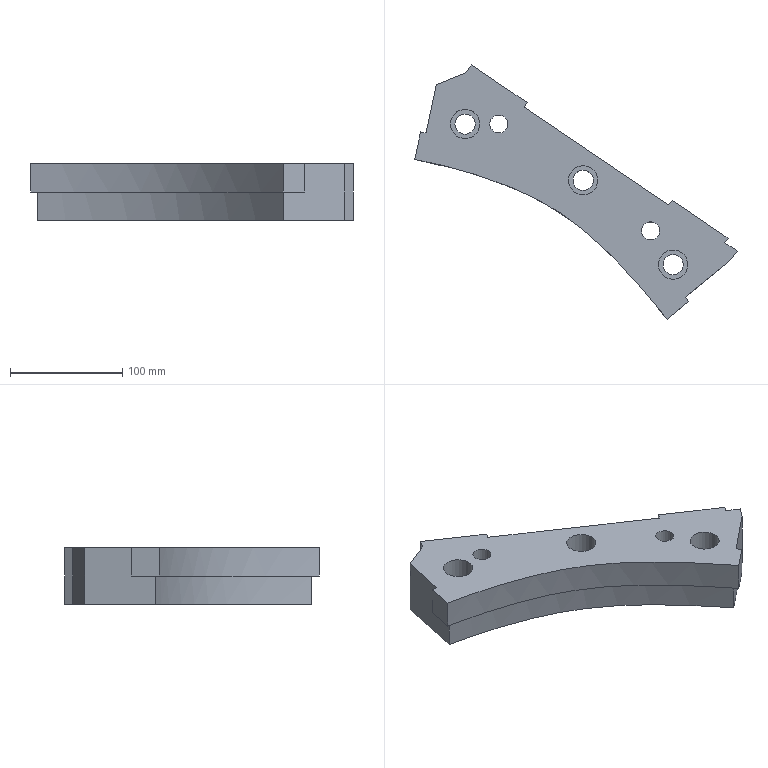Part | NX | features solid 2 | 1 solid | 32 faces | box 286.702 x 226.033 x 50 mm | volume 928298 mm3 | plane 20 | cylinder 8 | spline 4 | commonest cylinder face diameters 18 x3 26 x3 16 x2
STEP:
#1=CARTESIAN_POINT('',(-270.346,-232.178,0.));
#2=VERTEX_POINT('',#1);
#3=CARTESIAN_POINT('',(-275.25,-231.199,0.));
#4=VERTEX_POINT('',#3);
#5=CARTESIAN_POINT('',(-270.346,-232.178,0.));
#6=CARTESIAN_POINT('',(-271.979,-231.846,0.));
#7=CARTESIAN_POINT('',(-273.614,-231.52,0.));
#8=CARTESIAN_POINT('',(-275.25,-231.199,0.));
#9=B_SPLINE_CURVE_WITH_KNOTS('',3,(#5,#6,#7,#8),.UNSPECIFIED.,.F.,.F.,(4,4),(1.379,1.384),.UNSPECIFIED.);
#10=EDGE_CURVE('',#2,#4,#9,.T.);
#11=ORIENTED_EDGE('',*,*,#10,.F.);
#12=CARTESIAN_POINT('',(-270.346,-232.178,-25.));
#13=VERTEX_POINT('',#12);
#14=CARTESIAN_POINT('',(-270.346,-232.178,-25.));
#15=DIRECTION('',(0.,0.,-1.));
#16=VECTOR('',#15,1000.);
#17=LINE('',#14,#16);
#18=EDGE_CURVE('',#13,#2,#17,.F.);
#19=ORIENTED_EDGE('',*,*,#18,.F.);
#20=CARTESIAN_POINT('',(-275.25,-231.199,-25.));
#21=VERTEX_POINT('',#20);
#22=CARTESIAN_POINT('',(-270.346,-232.178,-25.));
#23=CARTESIAN_POINT('',(-271.981,-231.845,-25.));
#24=CARTESIAN_POINT('',(-273.615,-231.519,-25.));
#25=CARTESIAN_POINT('',(-275.25,-231.199,-25.));
#26=B_SPLINE_CURVE_WITH_KNOTS('',3,(#22,#23,#24,#25),.UNSPECIFIED.,.F.,.F.,(4,4),(0.9809,0.9985),.UNSPECIFIED.);
#27=EDGE_CURVE('',#13,#21,#26,.T.);
#28=ORIENTED_EDGE('',*,*,#27,.T.);
#29=CARTESIAN_POINT('',(-275.25,-231.199,-12.5));
#30=DIRECTION('',(0.,0.,-1.));
#31=VECTOR('',#30,1000.);
#32=LINE('',#29,#31);
#33=EDGE_CURVE('',#4,#21,#32,.T.);
#34=ORIENTED_EDGE('',*,*,#33,.F.);
#35=EDGE_LOOP('',(#11,#19,#28,#34));
#36=FACE_BOUND('',#35,.T.);
#37=CARTESIAN_POINT('',(-270.346,-232.178,0.));
#38=CARTESIAN_POINT('',(-270.346,-232.178,-25.));
#39=CARTESIAN_POINT('',(-271.981,-231.845,0.));
#40=CARTESIAN_POINT('',(-271.981,-231.845,-25.));
#41=CARTESIAN_POINT('',(-273.615,-231.519,0.));
#42=CARTESIAN_POINT('',(-273.615,-231.519,-25.));
#43=CARTESIAN_POINT('',(-275.25,-231.199,0.));
#44=CARTESIAN_POINT('',(-275.25,-231.199,-25.));
#45=B_SPLINE_SURFACE_WITH_KNOTS('',3,1,((#37,#38),(#39,#40),(#41,#42),(#43,#44)),.SURF_OF_LINEAR_EXTRUSION.,.F.,.F.,.F.,(4,4),(2,2),(0.9809,0.9985),(0.,1.),.PIECEWISE_BEZIER_KNOTS.);
#46=ADVANCED_FACE('',(#36),#45,.F.);
#47=CARTESIAN_POINT('',(-261.224,-189.264,-50.));
#48=VERTEX_POINT('',#47);
#49=CARTESIAN_POINT('',(-235.001,-178.669,-50.));
#50=VERTEX_POINT('',#49);
#51=CARTESIAN_POINT('',(-258.097,-188.001,-50.));
#52=DIRECTION('',(-0.9272,-0.3746,0.));
#53=VECTOR('',#52,1000.);
#54=LINE('',#51,#53);
#55=EDGE_CURVE('',#48,#50,#54,.F.);
#56=ORIENTED_EDGE('',*,*,#55,.T.);
#57=CARTESIAN_POINT('',(-230.246,-171.62,-50.));
#58=VERTEX_POINT('',#57);
#59=CARTESIAN_POINT('',(-224.654,-163.329,-50.));
#60=DIRECTION('',(0.5592,0.829,0.));
#61=VECTOR('',#60,1000.);
#62=LINE('',#59,#61);
#63=EDGE_CURVE('',#50,#58,#62,.T.);
#64=ORIENTED_EDGE('',*,*,#63,.T.);
#65=CARTESIAN_POINT('',(-180.503,-205.171,-50.));
#66=VERTEX_POINT('',#65);
#67=CARTESIAN_POINT('',(-72.1,-278.29,-50.));
#68=DIRECTION('',(0.829,-0.5592,0.));
#69=VECTOR('',#68,1000.);
#70=LINE('',#67,#69);
#71=EDGE_CURVE('',#58,#66,#70,.T.);
#72=ORIENTED_EDGE('',*,*,#71,.T.);
#73=CARTESIAN_POINT('',(-183.299,-209.317,-50.));
#74=VERTEX_POINT('',#73);
#75=CARTESIAN_POINT('',(-174.911,-196.881,-50.));
#76=DIRECTION('',(0.5592,0.829,0.));
#77=VECTOR('',#76,1000.);
#78=LINE('',#75,#77);
#79=EDGE_CURVE('',#74,#66,#78,.T.);
#80=ORIENTED_EDGE('',*,*,#79,.F.);
#81=CARTESIAN_POINT('',(-54.469,-296.214,-50.));
#82=VERTEX_POINT('',#81);
#83=CARTESIAN_POINT('',(-74.896,-282.435,-50.));
#84=DIRECTION('',(0.829,-0.5592,0.));
#85=VECTOR('',#84,1000.);
#86=LINE('',#83,#85);
#87=EDGE_CURVE('',#74,#82,#86,.T.);
#88=ORIENTED_EDGE('',*,*,#87,.T.);
#89=CARTESIAN_POINT('',(-51.673,-292.069,-50.));
#90=VERTEX_POINT('',#89);
#91=CARTESIAN_POINT('',(-46.081,-283.778,-50.));
#92=DIRECTION('',(0.5592,0.829,0.));
#93=VECTOR('',#92,1000.);
#94=LINE('',#91,#93);
#95=EDGE_CURVE('',#82,#90,#94,.T.);
#96=ORIENTED_EDGE('',*,*,#95,.T.);
#97=CARTESIAN_POINT('',(-1.931,-325.62,-50.));
#98=VERTEX_POINT('',#97);
#99=CARTESIAN_POINT('',(-72.1,-278.29,-50.));
#100=DIRECTION('',(0.829,-0.5592,0.));
#101=VECTOR('',#100,1000.);
#102=LINE('',#99,#101);
#103=EDGE_CURVE('',#90,#98,#102,.T.);
#104=ORIENTED_EDGE('',*,*,#103,.T.);
#105=CARTESIAN_POINT('',(-4.727,-329.765,-50.));
#106=VERTEX_POINT('',#105);
#107=CARTESIAN_POINT('',(3.661,-317.33,-50.));
#108=DIRECTION('',(0.5592,0.829,0.));
#109=VECTOR('',#108,1000.);
#110=LINE('',#107,#109);
#111=EDGE_CURVE('',#106,#98,#110,.T.);
#112=ORIENTED_EDGE('',*,*,#111,.F.);
#113=CARTESIAN_POINT('',(6.254,-337.172,-50.));
#114=VERTEX_POINT('',#113);
#115=CARTESIAN_POINT('',(-74.896,-282.435,-50.));
#116=DIRECTION('',(0.829,-0.5592,0.));
#117=VECTOR('',#116,1000.);
#118=LINE('',#115,#117);
#119=EDGE_CURVE('',#106,#114,#118,.T.);
#120=ORIENTED_EDGE('',*,*,#119,.T.);
#121=CARTESIAN_POINT('',(-1.187,-346.696,-50.));
#122=VERTEX_POINT('',#121);
#123=CARTESIAN_POINT('',(-528.329,-1021.407,-50.));
#124=DIRECTION('',(0.6157,0.788,0.));
#125=VECTOR('',#124,1000.);
#126=LINE('',#123,#125);
#127=EDGE_CURVE('',#122,#114,#126,.T.);
#128=ORIENTED_EDGE('',*,*,#127,.F.);
#129=CARTESIAN_POINT('',(-55.411,-390.605,-50.));
#130=VERTEX_POINT('',#129);
#131=CARTESIAN_POINT('',(-656.08,-877.018,-50.));
#132=DIRECTION('',(0.7771,0.6293,0.));
#133=VECTOR('',#132,1000.);
#134=LINE('',#131,#133);
#135=EDGE_CURVE('',#130,#122,#134,.T.);
#136=ORIENTED_EDGE('',*,*,#135,.F.);
#137=CARTESIAN_POINT('',(-274.504,-251.742,-50.));
#138=VERTEX_POINT('',#137);
#139=CARTESIAN_POINT('',(-55.411,-390.605,-50.));
#140=CARTESIAN_POINT('',(-57.422,-388.104,-50.));
#141=CARTESIAN_POINT('',(-61.329,-383.276,-50.));
#142=CARTESIAN_POINT('',(-65.923,-377.683,-50.));
#143=CARTESIAN_POINT('',(-69.426,-373.471,-50.));
#144=CARTESIAN_POINT('',(-71.964,-370.447,-50.));
#145=CARTESIAN_POINT('',(-74.015,-368.028,-50.));
#146=CARTESIAN_POINT('',(-75.397,-366.41,-50.));
#147=CARTESIAN_POINT('',(-76.201,-365.474,-50.));
#148=CARTESIAN_POINT('',(-76.728,-364.861,-50.));
#149=CARTESIAN_POINT('',(-77.518,-363.946,-50.));
#150=CARTESIAN_POINT('',(-78.477,-362.839,-50.));
#151=CARTESIAN_POINT('',(-80.191,-360.871,-50.));
#152=CARTESIAN_POINT('',(-82.598,-358.137,-50.));
#153=CARTESIAN_POINT('',(-85.465,-354.929,-50.));
#154=CARTESIAN_POINT('',(-89.243,-350.768,-50.));
#155=CARTESIAN_POINT('',(-92.968,-346.763,-50.));
#156=CARTESIAN_POINT('',(-96.153,-343.427,-50.));
#157=CARTESIAN_POINT('',(-97.989,-341.53,-50.));
#158=CARTESIAN_POINT('',(-99.27,-340.218,-50.));
#159=CARTESIAN_POINT('',(-100.882,-338.583,-50.));
#160=CARTESIAN_POINT('',(-102.912,-336.548,-50.));
#161=CARTESIAN_POINT('',(-106.509,-332.999,-50.));
#162=CARTESIAN_POINT('',(-111.59,-328.156,-50.));
#163=CARTESIAN_POINT('',(-116.654,-323.554,-50.));
#164=CARTESIAN_POINT('',(-120.161,-320.486,-50.));
#165=CARTESIAN_POINT('',(-122.185,-318.75,-50.));
#166=CARTESIAN_POINT('',(-123.628,-317.528,-50.));
#167=CARTESIAN_POINT('',(-125.348,-316.093,-50.));
#168=CARTESIAN_POINT('',(-127.548,-314.286,-50.));
#169=CARTESIAN_POINT('',(-131.451,-311.152,-50.));
#170=CARTESIAN_POINT('',(-137.03,-306.886,-50.));
#171=CARTESIAN_POINT('',(-142.64,-302.873,-50.));
#172=CARTESIAN_POINT('',(-147.169,-299.802,-50.));
#173=CARTESIAN_POINT('',(-150.51,-297.616,-50.));
#174=CARTESIAN_POINT('',(-154.112,-295.349,-50.));
#175=CARTESIAN_POINT('',(-157.69,-293.191,-50.));
#176=CARTESIAN_POINT('',(-161.299,-291.101,-50.));
#177=CARTESIAN_POINT('',(-165.002,-289.05,-50.));
#178=CARTESIAN_POINT('',(-168.496,-287.195,-50.));
#179=CARTESIAN_POINT('',(-172.17,-285.318,-50.));
#180=CARTESIAN_POINT('',(-175.308,-283.777,-50.));
#181=CARTESIAN_POINT('',(-177.846,-282.567,-50.));
#182=CARTESIAN_POINT('',(-179.85,-281.63,-50.));
#183=CARTESIAN_POINT('',(-181.587,-280.833,-50.));
#184=CARTESIAN_POINT('',(-184.022,-279.732,-50.));
#185=CARTESIAN_POINT('',(-188.293,-277.849,-50.));
#186=CARTESIAN_POINT('',(-194.575,-275.21,-50.));
#187=CARTESIAN_POINT('',(-201.05,-272.663,-50.));
#188=CARTESIAN_POINT('',(-205.707,-270.919,-50.));
#189=CARTESIAN_POINT('',(-208.377,-269.943,-50.));
#190=CARTESIAN_POINT('',(-210.458,-269.195,-50.));
#191=CARTESIAN_POINT('',(-212.314,-268.539,-50.));
#192=CARTESIAN_POINT('',(-214.883,-267.645,-50.));
#193=CARTESIAN_POINT('',(-219.375,-266.122,-50.));
#194=CARTESIAN_POINT('',(-225.901,-264.017,-50.));
#195=CARTESIAN_POINT('',(-232.566,-262.013,-50.));
#196=CARTESIAN_POINT('',(-237.931,-260.483,-50.));
#197=CARTESIAN_POINT('',(-242.113,-259.335,-50.));
#198=CARTESIAN_POINT('',(-245.872,-258.34,-50.));
#199=CARTESIAN_POINT('',(-251.127,-256.993,-50.));
#200=CARTESIAN_POINT('',(-260.442,-254.73,-50.));
#201=CARTESIAN_POINT('',(-268.793,-252.904,-50.));
#202=CARTESIAN_POINT('',(-274.504,-251.742,-50.));
#203=B_SPLINE_CURVE_WITH_KNOTS('',3,(#139,#140,#141,#142,#143,#144,#145,#146,#147,#148,#149,#150,#151,#152,#153,#154,#155,#156,#157,#158,#159,#160,#161,#162,#163,#164,#165,#166,#167,#168,#169,#170,#171,#172,#173,#174,#175,#176,#177,#178,#179,#180,#181,#182,#183,#184,#185,#186,#187,#188,#189,#190,#191,#192,#193,#194,#195,#196,#197,#198,#199,#200,#201,#202),.UNSPECIFIED.,.F.,.F.,(4,1,1,1,1,1,1,1,1,1,1,1,1,1,1,1,1,1,1,1,1,1,1,1,1,1,1,1,1,1,1,1,1,1,1,1,1,1,1,1,1,1,1,1,1,1,1,1,1,1,1,1,1,1,1,1,1,1,1,1,1,4),(0.,0.03125,0.0625,0.07812,0.09375,0.1094,0.1172,0.1211,0.125,0.1289,0.1328,0.1406,0.1562,0.1719,0.1875,0.2188,0.2344,0.2422,0.25,0.2578,0.2656,0.2812,0.3125,0.3438,0.3594,0.3672,0.375,0.3828,0.3906,0.4062,0.4375,0.4688,0.4844,0.5,0.5156,0.5312,0.5469,0.5625,0.5781,0.5938,0.6094,0.6172,0.625,0.6328,0.6406,0.6562,0.6875,0.7188,0.7344,0.7422,0.75,0.7578,0.7656,0.7812,0.8125,0.8438,0.8594,0.875,0.8906,0.9062,0.9375,1.),.UNSPECIFIED.);
#204=EDGE_CURVE('',#130,#138,#203,.T.);
#205=ORIENTED_EDGE('',*,*,#204,.T.);
#206=CARTESIAN_POINT('',(-438.593,-1023.717,-50.));
#207=DIRECTION('',(0.2079,0.9781,0.));
#208=VECTOR('',#207,1000.);
#209=LINE('',#206,#208);
#210=EDGE_CURVE('',#138,#48,#209,.T.);
#211=ORIENTED_EDGE('',*,*,#210,.T.);
#212=EDGE_LOOP('',(#56,#64,#72,#80,#88,#96,#104,#112,#120,#128,#136,#205,#211));
#213=FACE_BOUND('',#212,.T.);
#214=CARTESIAN_POINT('',(-62.718,-319.211,-50.));
#215=VERTEX_POINT('',#214);
#216=CARTESIAN_POINT('',(-70.718,-319.211,-50.));
#217=DIRECTION('',(0.,0.,1.));
#218=DIRECTION('',(1.,0.,0.));
#219=AXIS2_PLACEMENT_3D('',#216,#217,#218);
#220=CIRCLE('',#219,8.);
#221=EDGE_CURVE('',#215,#215,#220,.F.);
#222=ORIENTED_EDGE('',*,*,#221,.F.);
#223=EDGE_LOOP('',(#222));
#224=FACE_BOUND('',#223,.T.);
#225=CARTESIAN_POINT('',(-197.718,-224.211,-50.));
#226=VERTEX_POINT('',#225);
#227=CARTESIAN_POINT('',(-205.718,-224.211,-50.));
#228=DIRECTION('',(0.,0.,1.));
#229=DIRECTION('',(1.,0.,0.));
#230=AXIS2_PLACEMENT_3D('',#227,#228,#229);
#231=CIRCLE('',#230,8.);
#232=EDGE_CURVE('',#226,#226,#231,.F.);
#233=ORIENTED_EDGE('',*,*,#232,.F.);
#234=EDGE_LOOP('',(#233));
#235=FACE_BOUND('',#234,.T.);
#236=CARTESIAN_POINT('',(-226.718,-224.211,-50.));
#237=VERTEX_POINT('',#236);
#238=CARTESIAN_POINT('',(-235.718,-224.211,-50.));
#239=DIRECTION('',(0.,0.,1.));
#240=DIRECTION('',(1.,0.,0.));
#241=AXIS2_PLACEMENT_3D('',#238,#239,#240);
#242=CIRCLE('',#241,9.);
#243=EDGE_CURVE('',#237,#237,#242,.F.);
#244=ORIENTED_EDGE('',*,*,#243,.F.);
#245=EDGE_LOOP('',(#244));
#246=FACE_BOUND('',#245,.T.);
#247=CARTESIAN_POINT('',(-121.718,-274.211,-50.));
#248=VERTEX_POINT('',#247);
#249=CARTESIAN_POINT('',(-130.718,-274.211,-50.));
#250=DIRECTION('',(0.,0.,1.));
#251=DIRECTION('',(1.,0.,0.));
#252=AXIS2_PLACEMENT_3D('',#249,#250,#251);
#253=CIRCLE('',#252,9.);
#254=EDGE_CURVE('',#248,#248,#253,.F.);
#255=ORIENTED_EDGE('',*,*,#254,.F.);
#256=EDGE_LOOP('',(#255));
#257=FACE_BOUND('',#256,.T.);
#258=CARTESIAN_POINT('',(-41.718,-349.211,-50.));
#259=VERTEX_POINT('',#258);
#260=CARTESIAN_POINT('',(-50.718,-349.211,-50.));
#261=DIRECTION('',(0.,0.,1.));
#262=DIRECTION('',(1.,0.,0.));
#263=AXIS2_PLACEMENT_3D('',#260,#261,#262);
#264=CIRCLE('',#263,9.);
#265=EDGE_CURVE('',#259,#259,#264,.F.);
#266=ORIENTED_EDGE('',*,*,#265,.F.);
#267=EDGE_LOOP('',(#266));
#268=FACE_BOUND('',#267,.T.);
#269=CARTESIAN_POINT('',(-557.805,-998.377,-50.));
#270=DIRECTION('',(0.,0.,1.));
#271=DIRECTION('',(1.,0.,0.));
#272=AXIS2_PLACEMENT_3D('',#269,#270,#271);
#273=PLANE('',#272);
#274=ADVANCED_FACE('',(#213,#224,#235,#246,#257,#268),#273,.F.);
#275=ORIENTED_EDGE('',*,*,#87,.F.);
#276=CARTESIAN_POINT('',(-183.299,-209.317,0.));
#277=VERTEX_POINT('',#276);
#278=CARTESIAN_POINT('',(-183.299,-209.317,-25.));
#279=DIRECTION('',(0.,0.,-1.));
#280=VECTOR('',#279,1000.);
#281=LINE('',#278,#280);
#282=EDGE_CURVE('',#277,#74,#281,.T.);
#283=ORIENTED_EDGE('',*,*,#282,.F.);
#284=CARTESIAN_POINT('',(-54.469,-296.214,0.));
#285=VERTEX_POINT('',#284);
#286=CARTESIAN_POINT('',(-278.599,-145.036,0.));
#287=DIRECTION('',(-0.829,0.5592,0.));
#288=VECTOR('',#287,1000.);
#289=LINE('',#286,#288);
#290=EDGE_CURVE('',#285,#277,#289,.T.);
#291=ORIENTED_EDGE('',*,*,#290,.F.);
#292=CARTESIAN_POINT('',(-54.469,-296.214,-25.));
#293=DIRECTION('',(0.,0.,-1.));
#294=VECTOR('',#293,1000.);
#295=LINE('',#292,#294);
#296=EDGE_CURVE('',#285,#82,#295,.T.);
#297=ORIENTED_EDGE('',*,*,#296,.T.);
#298=EDGE_LOOP('',(#275,#283,#291,#297));
#299=FACE_BOUND('',#298,.T.);
#300=CARTESIAN_POINT('',(-278.599,-145.036,-70.));
#301=DIRECTION('',(-0.5592,-0.829,0.));
#302=DIRECTION('',(0.829,-0.5592,0.));
#303=AXIS2_PLACEMENT_3D('',#300,#301,#302);
#304=PLANE('',#303);
#305=ADVANCED_FACE('',(#299),#304,.F.);
#306=ORIENTED_EDGE('',*,*,#135,.T.);
#307=CARTESIAN_POINT('',(-1.187,-346.696,0.));
#308=VERTEX_POINT('',#307);
#309=CARTESIAN_POINT('',(-1.187,-346.696,-5.));
#310=DIRECTION('',(0.,0.,-1.));
#311=VECTOR('',#310,1000.);
#312=LINE('',#309,#311);
#313=EDGE_CURVE('',#308,#122,#312,.T.);
#314=ORIENTED_EDGE('',*,*,#313,.F.);
#315=CARTESIAN_POINT('',(-39.868,-378.019,0.));
#316=VERTEX_POINT('',#315);
#317=CARTESIAN_POINT('',(-59.315,-393.767,0.));
#318=DIRECTION('',(0.7771,0.6293,0.));
#319=VECTOR('',#318,1000.);
#320=LINE('',#317,#319);
#321=EDGE_CURVE('',#316,#308,#320,.T.);
#322=ORIENTED_EDGE('',*,*,#321,.F.);
#323=CARTESIAN_POINT('',(-39.868,-378.019,-25.));
#324=VERTEX_POINT('',#323);
#325=CARTESIAN_POINT('',(-39.868,-378.019,-25.));
#326=DIRECTION('',(0.,0.,-1.));
#327=VECTOR('',#326,1000.);
#328=LINE('',#325,#327);
#329=EDGE_CURVE('',#324,#316,#328,.F.);
#330=ORIENTED_EDGE('',*,*,#329,.F.);
#331=CARTESIAN_POINT('',(-55.411,-390.605,-25.));
#332=VERTEX_POINT('',#331);
#333=CARTESIAN_POINT('',(-55.43,-390.621,-25.));
#334=DIRECTION('',(0.7771,0.6293,0.));
#335=VECTOR('',#334,1000.);
#336=LINE('',#333,#335);
#337=EDGE_CURVE('',#332,#324,#336,.T.);
#338=ORIENTED_EDGE('',*,*,#337,.F.);
#339=CARTESIAN_POINT('',(-55.411,-390.605,-42.5));
#340=DIRECTION('',(0.,0.,1.));
#341=VECTOR('',#340,1000.);
#342=LINE('',#339,#341);
#343=EDGE_CURVE('',#332,#130,#342,.F.);
#344=ORIENTED_EDGE('',*,*,#343,.T.);
#345=EDGE_LOOP('',(#306,#314,#322,#330,#338,#344));
#346=FACE_BOUND('',#345,.T.);
#347=CARTESIAN_POINT('',(-55.43,-390.621,-70.));
#348=DIRECTION('',(0.6293,-0.7771,0.));
#349=DIRECTION('',(0.7771,0.6293,0.));
#350=AXIS2_PLACEMENT_3D('',#347,#348,#349);
#351=PLANE('',#350);
#352=ADVANCED_FACE('',(#346),#351,.T.);
#353=ORIENTED_EDGE('',*,*,#119,.F.);
#354=CARTESIAN_POINT('',(-4.727,-329.765,0.));
#355=VERTEX_POINT('',#354);
#356=CARTESIAN_POINT('',(-4.727,-329.765,-25.));
#357=DIRECTION('',(0.,0.,-1.));
#358=VECTOR('',#357,1000.);
#359=LINE('',#356,#358);
#360=EDGE_CURVE('',#355,#106,#359,.T.);
#361=ORIENTED_EDGE('',*,*,#360,.F.);
#362=CARTESIAN_POINT('',(6.254,-337.172,0.));
#363=VERTEX_POINT('',#362);
#364=CARTESIAN_POINT('',(-278.599,-145.036,0.));
#365=DIRECTION('',(-0.829,0.5592,0.));
#366=VECTOR('',#365,1000.);
#367=LINE('',#364,#366);
#368=EDGE_CURVE('',#363,#355,#367,.T.);
#369=ORIENTED_EDGE('',*,*,#368,.F.);
#370=CARTESIAN_POINT('',(6.254,-337.172,-70.));
#371=DIRECTION('',(0.,0.,1.));
#372=VECTOR('',#371,1000.);
#373=LINE('',#370,#372);
#374=EDGE_CURVE('',#114,#363,#373,.T.);
#375=ORIENTED_EDGE('',*,*,#374,.F.);
#376=EDGE_LOOP('',(#353,#361,#369,#375));
#377=FACE_BOUND('',#376,.T.);
#378=CARTESIAN_POINT('',(-278.599,-145.036,-70.));
#379=DIRECTION('',(-0.5592,-0.829,0.));
#380=DIRECTION('',(0.829,-0.5592,0.));
#381=AXIS2_PLACEMENT_3D('',#378,#379,#380);
#382=PLANE('',#381);
#383=ADVANCED_FACE('',(#377),#382,.F.);
#384=CARTESIAN_POINT('',(-261.224,-189.264,0.));
#385=VERTEX_POINT('',#384);
#386=CARTESIAN_POINT('',(-274.518,-251.805,0.));
#387=DIRECTION('',(-0.2079,-0.9781,0.));
#388=VECTOR('',#387,1000.);
#389=LINE('',#386,#388);
#390=EDGE_CURVE('',#385,#2,#389,.T.);
#391=ORIENTED_EDGE('',*,*,#390,.F.);
#392=CARTESIAN_POINT('',(-261.224,-189.264,-70.));
#393=DIRECTION('',(0.,0.,1.));
#394=VECTOR('',#393,1000.);
#395=LINE('',#392,#394);
#396=EDGE_CURVE('',#385,#48,#395,.F.);
#397=ORIENTED_EDGE('',*,*,#396,.T.);
#398=ORIENTED_EDGE('',*,*,#210,.F.);
#399=CARTESIAN_POINT('',(-274.504,-251.742,-25.));
#400=VERTEX_POINT('',#399);
#401=CARTESIAN_POINT('',(-274.504,-251.742,-42.5));
#402=DIRECTION('',(0.,0.,1.));
#403=VECTOR('',#402,1000.);
#404=LINE('',#401,#403);
#405=EDGE_CURVE('',#400,#138,#404,.F.);
#406=ORIENTED_EDGE('',*,*,#405,.F.);
#407=CARTESIAN_POINT('',(-274.518,-251.805,-25.));
#408=DIRECTION('',(0.2079,0.9781,0.));
#409=VECTOR('',#408,1000.);
#410=LINE('',#407,#409);
#411=EDGE_CURVE('',#400,#13,#410,.T.);
#412=ORIENTED_EDGE('',*,*,#411,.T.);
#413=ORIENTED_EDGE('',*,*,#18,.T.);
#414=EDGE_LOOP('',(#391,#397,#398,#406,#412,#413));
#415=FACE_BOUND('',#414,.T.);
#416=CARTESIAN_POINT('',(-274.518,-251.805,-70.));
#417=DIRECTION('',(0.9781,-0.2079,0.));
#418=DIRECTION('',(0.2079,0.9781,0.));
#419=AXIS2_PLACEMENT_3D('',#416,#417,#418);
#420=PLANE('',#419);
#421=ADVANCED_FACE('',(#415),#420,.F.);
#422=CARTESIAN_POINT('',(-55.411,-390.605,-25.));
#423=CARTESIAN_POINT('',(-62.399,-381.913,-25.));
#424=CARTESIAN_POINT('',(-76.555,-364.64,-25.));
#425=CARTESIAN_POINT('',(-98.928,-339.944,-25.));
#426=CARTESIAN_POINT('',(-119.078,-320.953,-25.));
#427=CARTESIAN_POINT('',(-136.462,-307.138,-25.));
#428=CARTESIAN_POINT('',(-150.294,-297.527,-25.));
#429=CARTESIAN_POINT('',(-164.763,-288.963,-25.));
#430=CARTESIAN_POINT('',(-179.626,-281.57,-25.));
#431=CARTESIAN_POINT('',(-194.833,-275.02,-25.));
#432=CARTESIAN_POINT('',(-215.448,-267.169,-25.));
#433=CARTESIAN_POINT('',(-241.844,-258.996,-25.));
#434=CARTESIAN_POINT('',(-263.581,-253.963,-25.));
#435=CARTESIAN_POINT('',(-274.504,-251.742,-25.));
#436=B_SPLINE_CURVE_WITH_KNOTS('',3,(#422,#423,#424,#425,#426,#427,#428,#429,#430,#431,#432,#433,#434,#435),.UNSPECIFIED.,.F.,.F.,(4,1,1,1,1,1,1,1,1,1,1,4),(1.098,1.131,1.165,1.198,1.215,1.232,1.249,1.265,1.282,1.299,1.332,1.366),.UNSPECIFIED.);
#437=EDGE_CURVE('',#332,#400,#436,.T.);
#438=ORIENTED_EDGE('',*,*,#437,.T.);
#439=ORIENTED_EDGE('',*,*,#405,.T.);
#440=ORIENTED_EDGE('',*,*,#204,.F.);
#441=ORIENTED_EDGE('',*,*,#343,.F.);
#442=EDGE_LOOP('',(#438,#439,#440,#441));
#443=FACE_BOUND('',#442,.T.);
#444=CARTESIAN_POINT('',(-55.411,-390.605,-50.));
#445=CARTESIAN_POINT('',(-55.411,-390.605,-25.));
#446=CARTESIAN_POINT('',(-69.194,-373.462,-50.));
#447=CARTESIAN_POINT('',(-69.194,-373.462,-25.));
#448=CARTESIAN_POINT('',(-90.451,-347.991,-50.));
#449=CARTESIAN_POINT('',(-90.451,-347.991,-25.));
#450=CARTESIAN_POINT('',(-122.802,-317.404,-50.));
#451=CARTESIAN_POINT('',(-122.802,-317.404,-25.));
#452=CARTESIAN_POINT('',(-145.193,-300.574,-50.));
#453=CARTESIAN_POINT('',(-145.193,-300.574,-25.));
#454=CARTESIAN_POINT('',(-164.483,-289.111,-50.));
#455=CARTESIAN_POINT('',(-164.483,-289.111,-25.));
#456=CARTESIAN_POINT('',(-179.491,-281.628,-50.));
#457=CARTESIAN_POINT('',(-179.491,-281.628,-25.));
#458=CARTESIAN_POINT('',(-194.824,-275.022,-50.));
#459=CARTESIAN_POINT('',(-194.824,-275.022,-25.));
#460=CARTESIAN_POINT('',(-215.584,-267.118,-50.));
#461=CARTESIAN_POINT('',(-215.584,-267.118,-25.));
#462=CARTESIAN_POINT('',(-242.101,-258.929,-50.));
#463=CARTESIAN_POINT('',(-242.101,-258.929,-25.));
#464=CARTESIAN_POINT('',(-263.671,-253.945,-50.));
#465=CARTESIAN_POINT('',(-263.671,-253.945,-25.));
#466=CARTESIAN_POINT('',(-274.504,-251.742,-50.));
#467=CARTESIAN_POINT('',(-274.504,-251.742,-25.));
#468=B_SPLINE_SURFACE_WITH_KNOTS('',3,1,((#444,#445),(#446,#447),(#448,#449),(#450,#451),(#452,#453),(#454,#455),(#456,#457),(#458,#459),(#460,#461),(#462,#463),(#464,#465),(#466,#467)),.SURF_OF_LINEAR_EXTRUSION.,.F.,.F.,.F.,(4,1,1,1,1,1,1,1,1,4),(2,2),(0.01836,0.2592,0.3796,0.5,0.5601,0.6203,0.6805,0.7407,0.8611,0.9815),(0.,1.),.UNSPECIFIED.);
#469=ADVANCED_FACE('',(#443),#468,.F.);
#470=CARTESIAN_POINT('',(-280.448,-255.656,0.));
#471=VERTEX_POINT('',#470);
#472=CARTESIAN_POINT('',(-443.483,-1022.677,0.));
#473=DIRECTION('',(0.2079,0.9781,0.));
#474=VECTOR('',#473,1000.);
#475=LINE('',#472,#474);
#476=EDGE_CURVE('',#471,#4,#475,.T.);
#477=ORIENTED_EDGE('',*,*,#476,.T.);
#478=ORIENTED_EDGE('',*,*,#33,.T.);
#479=CARTESIAN_POINT('',(-280.448,-255.656,-25.));
#480=VERTEX_POINT('',#479);
#481=CARTESIAN_POINT('',(-578.39,-1657.361,-25.));
#482=DIRECTION('',(0.2079,0.9781,0.));
#483=VECTOR('',#482,1000.);
#484=LINE('',#481,#483);
#485=EDGE_CURVE('',#480,#21,#484,.T.);
#486=ORIENTED_EDGE('',*,*,#485,.F.);
#487=CARTESIAN_POINT('',(-280.448,-255.656,-30.));
#488=DIRECTION('',(0.,0.,1.));
#489=VECTOR('',#488,1000.);
#490=LINE('',#487,#489);
#491=EDGE_CURVE('',#480,#471,#490,.T.);
#492=ORIENTED_EDGE('',*,*,#491,.T.);
#493=EDGE_LOOP('',(#477,#478,#486,#492));
#494=FACE_BOUND('',#493,.T.);
#495=CARTESIAN_POINT('',(-578.39,-1657.361,-70.));
#496=DIRECTION('',(0.9781,-0.2079,0.));
#497=DIRECTION('',(0.2079,0.9781,0.));
#498=AXIS2_PLACEMENT_3D('',#495,#496,#497);
#499=PLANE('',#498);
#500=ADVANCED_FACE('',(#494),#499,.F.);
#501=CARTESIAN_POINT('',(-56.169,-397.653,-25.));
#502=VERTEX_POINT('',#501);
#503=CARTESIAN_POINT('',(-280.448,-255.656,-25.));
#504=CARTESIAN_POINT('',(-269.382,-257.815,-25.));
#505=CARTESIAN_POINT('',(-247.347,-262.708,-25.));
#506=CARTESIAN_POINT('',(-220.183,-270.825,-25.));
#507=CARTESIAN_POINT('',(-198.674,-278.853,-25.));
#508=CARTESIAN_POINT('',(-182.82,-285.591,-25.));
#509=CARTESIAN_POINT('',(-167.429,-293.185,-25.));
#510=CARTESIAN_POINT('',(-152.575,-301.988,-25.));
#511=CARTESIAN_POINT('',(-138.48,-311.859,-25.));
#512=CARTESIAN_POINT('',(-120.792,-326.083,-25.));
#513=CARTESIAN_POINT('',(-100.348,-345.642,-25.));
#514=CARTESIAN_POINT('',(-77.669,-371.038,-25.));
#515=CARTESIAN_POINT('',(-63.29,-388.75,-25.));
#516=CARTESIAN_POINT('',(-56.169,-397.653,-25.));
#517=B_SPLINE_CURVE_WITH_KNOTS('',3,(#503,#504,#505,#506,#507,#508,#509,#510,#511,#512,#513,#514,#515,#516),.UNSPECIFIED.,.F.,.F.,(4,1,1,1,1,1,1,1,1,1,1,4),(0.9116,0.9455,0.9794,0.9963,1.013,1.03,1.047,1.064,1.081,1.115,1.149,1.183),.UNSPECIFIED.);
#518=EDGE_CURVE('',#502,#480,#517,.F.);
#519=ORIENTED_EDGE('',*,*,#518,.F.);
#520=CARTESIAN_POINT('',(-56.169,-397.653,0.));
#521=VERTEX_POINT('',#520);
#522=CARTESIAN_POINT('',(-56.169,-397.653,-70.));
#523=DIRECTION('',(0.,0.,1.));
#524=VECTOR('',#523,1000.);
#525=LINE('',#522,#524);
#526=EDGE_CURVE('',#502,#521,#525,.T.);
#527=ORIENTED_EDGE('',*,*,#526,.T.);
#528=CARTESIAN_POINT('',(-56.169,-397.653,0.));
#529=CARTESIAN_POINT('',(-63.276,-388.767,0.));
#530=CARTESIAN_POINT('',(-77.625,-371.093,0.));
#531=CARTESIAN_POINT('',(-100.228,-345.769,0.));
#532=CARTESIAN_POINT('',(-124.653,-322.383,0.));
#533=CARTESIAN_POINT('',(-147.129,-305.265,0.));
#534=CARTESIAN_POINT('',(-166.987,-293.42,0.));
#535=CARTESIAN_POINT('',(-182.401,-285.784,0.));
#536=CARTESIAN_POINT('',(-198.132,-279.072,0.));
#537=CARTESIAN_POINT('',(-219.459,-271.069,0.));
#538=CARTESIAN_POINT('',(-246.749,-262.849,0.));
#539=CARTESIAN_POINT('',(-269.194,-257.852,0.));
#540=CARTESIAN_POINT('',(-280.448,-255.656,0.));
#541=B_SPLINE_CURVE_WITH_KNOTS('',3,(#528,#529,#530,#531,#532,#533,#534,#535,#536,#537,#538,#539,#540),.UNSPECIFIED.,.F.,.F.,(4,1,1,1,1,1,1,1,1,1,4),(1.525,1.557,1.589,1.622,1.654,1.67,1.686,1.702,1.718,1.75,1.782),.UNSPECIFIED.);
#542=EDGE_CURVE('',#521,#471,#541,.T.);
#543=ORIENTED_EDGE('',*,*,#542,.T.);
#544=ORIENTED_EDGE('',*,*,#491,.F.);
#545=EDGE_LOOP('',(#519,#527,#543,#544));
#546=FACE_BOUND('',#545,.T.);
#547=CARTESIAN_POINT('',(-56.169,-397.653,-25.));
#548=CARTESIAN_POINT('',(-56.169,-397.653,0.));
#549=CARTESIAN_POINT('',(-70.391,-379.87,-25.));
#550=CARTESIAN_POINT('',(-70.391,-379.87,0.));
#551=CARTESIAN_POINT('',(-92.144,-353.476,-25.));
#552=CARTESIAN_POINT('',(-92.144,-353.476,0.));
#553=CARTESIAN_POINT('',(-125.076,-321.991,-25.));
#554=CARTESIAN_POINT('',(-125.076,-321.991,0.));
#555=CARTESIAN_POINT('',(-147.839,-304.789,-25.));
#556=CARTESIAN_POINT('',(-147.839,-304.789,0.));
#557=CARTESIAN_POINT('',(-167.425,-293.192,-25.));
#558=CARTESIAN_POINT('',(-167.425,-293.192,0.));
#559=CARTESIAN_POINT('',(-182.736,-285.631,-25.));
#560=CARTESIAN_POINT('',(-182.736,-285.631,0.));
#561=CARTESIAN_POINT('',(-198.461,-278.94,-25.));
#562=CARTESIAN_POINT('',(-198.461,-278.94,0.));
#563=CARTESIAN_POINT('',(-219.786,-270.96,-25.));
#564=CARTESIAN_POINT('',(-219.786,-270.96,0.));
#565=CARTESIAN_POINT('',(-247.041,-262.779,-25.));
#566=CARTESIAN_POINT('',(-247.041,-262.779,0.));
#567=CARTESIAN_POINT('',(-269.273,-257.836,-25.));
#568=CARTESIAN_POINT('',(-269.273,-257.836,0.));
#569=CARTESIAN_POINT('',(-280.448,-255.656,-25.));
#570=CARTESIAN_POINT('',(-280.448,-255.656,0.));
#571=B_SPLINE_SURFACE_WITH_KNOTS('',3,1,((#547,#548),(#549,#550),(#551,#552),(#553,#554),(#555,#556),(#557,#558),(#559,#560),(#561,#562),(#563,#564),(#565,#566),(#567,#568),(#569,#570)),.SURF_OF_LINEAR_EXTRUSION.,.F.,.F.,.F.,(4,1,1,1,1,1,1,1,1,4),(2,2),(0.258,0.3163,0.3454,0.3746,0.3891,0.4037,0.4183,0.4328,0.462,0.4911),(0.,1.),.UNSPECIFIED.);
#572=ADVANCED_FACE('',(#546),#571,.F.);
#573=CARTESIAN_POINT('',(-36.74,-381.92,0.));
#574=VERTEX_POINT('',#573);
#575=CARTESIAN_POINT('',(-36.74,-381.92,-25.));
#576=VERTEX_POINT('',#575);
#577=CARTESIAN_POINT('',(-36.74,-381.92,-12.5));
#578=DIRECTION('',(0.,0.,-1.));
#579=VECTOR('',#578,1000.);
#580=LINE('',#577,#579);
#581=EDGE_CURVE('',#574,#576,#580,.T.);
#582=ORIENTED_EDGE('',*,*,#581,.F.);
#583=CARTESIAN_POINT('',(-652.933,-880.903,0.));
#584=DIRECTION('',(0.7771,0.6293,0.));
#585=VECTOR('',#584,1000.);
#586=LINE('',#583,#585);
#587=EDGE_CURVE('',#521,#574,#586,.T.);
#588=ORIENTED_EDGE('',*,*,#587,.F.);
#589=ORIENTED_EDGE('',*,*,#526,.F.);
#590=CARTESIAN_POINT('',(-1585.628,-1636.184,-25.));
#591=DIRECTION('',(0.7771,0.6293,0.));
#592=VECTOR('',#591,1000.);
#593=LINE('',#590,#592);
#594=EDGE_CURVE('',#502,#576,#593,.T.);
#595=ORIENTED_EDGE('',*,*,#594,.T.);
#596=EDGE_LOOP('',(#582,#588,#589,#595));
#597=FACE_BOUND('',#596,.T.);
#598=CARTESIAN_POINT('',(-1585.628,-1636.184,-70.));
#599=DIRECTION('',(0.6293,-0.7771,0.));
#600=DIRECTION('',(0.7771,0.6293,0.));
#601=AXIS2_PLACEMENT_3D('',#598,#599,#600);
#602=PLANE('',#601);
#603=ADVANCED_FACE('',(#597),#602,.T.);
#604=ORIENTED_EDGE('',*,*,#10,.T.);
#605=ORIENTED_EDGE('',*,*,#476,.F.);
#606=ORIENTED_EDGE('',*,*,#542,.F.);
#607=ORIENTED_EDGE('',*,*,#587,.T.);
#608=CARTESIAN_POINT('',(-36.74,-381.92,0.));
#609=CARTESIAN_POINT('',(-37.781,-380.618,0.));
#610=CARTESIAN_POINT('',(-38.823,-379.318,0.));
#611=CARTESIAN_POINT('',(-39.868,-378.019,0.));
#612=B_SPLINE_CURVE_WITH_KNOTS('',3,(#608,#609,#610,#611),.UNSPECIFIED.,.F.,.F.,(4,4),(1.093,1.098),.UNSPECIFIED.);
#613=EDGE_CURVE('',#574,#316,#612,.T.);
#614=ORIENTED_EDGE('',*,*,#613,.T.);
#615=ORIENTED_EDGE('',*,*,#321,.T.);
#616=CARTESIAN_POINT('',(-46.749,-405.013,0.));
#617=DIRECTION('',(0.6157,0.788,0.));
#618=VECTOR('',#617,1000.);
#619=LINE('',#616,#618);
#620=EDGE_CURVE('',#308,#363,#619,.T.);
#621=ORIENTED_EDGE('',*,*,#620,.T.);
#622=ORIENTED_EDGE('',*,*,#368,.T.);
#623=CARTESIAN_POINT('',(-1.931,-325.62,0.));
#624=VERTEX_POINT('',#623);
#625=CARTESIAN_POINT('',(-52.284,-400.273,0.));
#626=DIRECTION('',(0.5592,0.829,0.));
#627=VECTOR('',#626,1000.);
#628=LINE('',#625,#627);
#629=EDGE_CURVE('',#355,#624,#628,.T.);
#630=ORIENTED_EDGE('',*,*,#629,.T.);
#631=CARTESIAN_POINT('',(-51.673,-292.069,0.));
#632=VERTEX_POINT('',#631);
#633=CARTESIAN_POINT('',(-72.1,-278.29,0.));
#634=DIRECTION('',(0.829,-0.5592,0.));
#635=VECTOR('',#634,1000.);
#636=LINE('',#633,#635);
#637=EDGE_CURVE('',#632,#624,#636,.T.);
#638=ORIENTED_EDGE('',*,*,#637,.F.);
#639=CARTESIAN_POINT('',(-102.027,-366.721,0.));
#640=DIRECTION('',(0.5592,0.829,0.));
#641=VECTOR('',#640,1000.);
#642=LINE('',#639,#641);
#643=EDGE_CURVE('',#285,#632,#642,.T.);
#644=ORIENTED_EDGE('',*,*,#643,.F.);
#645=ORIENTED_EDGE('',*,*,#290,.T.);
#646=CARTESIAN_POINT('',(-180.503,-205.171,0.));
#647=VERTEX_POINT('',#646);
#648=CARTESIAN_POINT('',(-230.857,-279.824,0.));
#649=DIRECTION('',(0.5592,0.829,0.));
#650=VECTOR('',#649,1000.);
#651=LINE('',#648,#650);
#652=EDGE_CURVE('',#277,#647,#651,.T.);
#653=ORIENTED_EDGE('',*,*,#652,.T.);
#654=CARTESIAN_POINT('',(-230.246,-171.62,0.));
#655=VERTEX_POINT('',#654);
#656=CARTESIAN_POINT('',(-72.1,-278.29,0.));
#657=DIRECTION('',(0.829,-0.5592,0.));
#658=VECTOR('',#657,1000.);
#659=LINE('',#656,#658);
#660=EDGE_CURVE('',#655,#647,#659,.T.);
#661=ORIENTED_EDGE('',*,*,#660,.F.);
#662=CARTESIAN_POINT('',(-235.001,-178.669,0.));
#663=VERTEX_POINT('',#662);
#664=CARTESIAN_POINT('',(-280.6,-246.273,0.));
#665=DIRECTION('',(0.5592,0.829,0.));
#666=VECTOR('',#665,1000.);
#667=LINE('',#664,#666);
#668=EDGE_CURVE('',#663,#655,#667,.T.);
#669=ORIENTED_EDGE('',*,*,#668,.F.);
#670=CARTESIAN_POINT('',(-797.214,-405.818,0.));
#671=DIRECTION('',(0.9272,0.3746,0.));
#672=VECTOR('',#671,1000.);
#673=LINE('',#670,#672);
#674=EDGE_CURVE('',#663,#385,#673,.F.);
#675=ORIENTED_EDGE('',*,*,#674,.T.);
#676=ORIENTED_EDGE('',*,*,#390,.T.);
#677=EDGE_LOOP('',(#604,#605,#606,#607,#614,#615,#621,#622,#630,#638,#644,#645,#653,#661,#669,#675,#676));
#678=FACE_BOUND('',#677,.T.);
#679=CARTESIAN_POINT('',(-117.718,-274.211,0.));
#680=VERTEX_POINT('',#679);
#681=CARTESIAN_POINT('',(-130.718,-274.211,0.));
#682=DIRECTION('',(0.,0.,1.));
#683=DIRECTION('',(1.,0.,0.));
#684=AXIS2_PLACEMENT_3D('',#681,#682,#683);
#685=CIRCLE('',#684,13.);
#686=EDGE_CURVE('',#680,#680,#685,.F.);
#687=ORIENTED_EDGE('',*,*,#686,.T.);
#688=EDGE_LOOP('',(#687));
#689=FACE_BOUND('',#688,.T.);
#690=CARTESIAN_POINT('',(-197.718,-224.211,0.));
#691=VERTEX_POINT('',#690);
#692=CARTESIAN_POINT('',(-205.718,-224.211,0.));
#693=DIRECTION('',(0.,0.,1.));
#694=DIRECTION('',(1.,0.,0.));
#695=AXIS2_PLACEMENT_3D('',#692,#693,#694);
#696=CIRCLE('',#695,8.);
#697=EDGE_CURVE('',#691,#691,#696,.F.);
#698=ORIENTED_EDGE('',*,*,#697,.T.);
#699=EDGE_LOOP('',(#698));
#700=FACE_BOUND('',#699,.T.);
#701=CARTESIAN_POINT('',(-62.718,-319.211,0.));
#702=VERTEX_POINT('',#701);
#703=CARTESIAN_POINT('',(-70.718,-319.211,0.));
#704=DIRECTION('',(0.,0.,1.));
#705=DIRECTION('',(1.,0.,0.));
#706=AXIS2_PLACEMENT_3D('',#703,#704,#705);
#707=CIRCLE('',#706,8.);
#708=EDGE_CURVE('',#702,#702,#707,.F.);
#709=ORIENTED_EDGE('',*,*,#708,.T.);
#710=EDGE_LOOP('',(#709));
#711=FACE_BOUND('',#710,.T.);
#712=CARTESIAN_POINT('',(-222.718,-224.211,0.));
#713=VERTEX_POINT('',#712);
#714=CARTESIAN_POINT('',(-235.718,-224.211,0.));
#715=DIRECTION('',(0.,0.,1.));
#716=DIRECTION('',(1.,0.,0.));
#717=AXIS2_PLACEMENT_3D('',#714,#715,#716);
#718=CIRCLE('',#717,13.);
#719=EDGE_CURVE('',#713,#713,#718,.F.);
#720=ORIENTED_EDGE('',*,*,#719,.T.);
#721=EDGE_LOOP('',(#720));
#722=FACE_BOUND('',#721,.T.);
#723=CARTESIAN_POINT('',(-37.718,-349.211,0.));
#724=VERTEX_POINT('',#723);
#725=CARTESIAN_POINT('',(-50.718,-349.211,0.));
#726=DIRECTION('',(0.,0.,1.));
#727=DIRECTION('',(1.,0.,0.));
#728=AXIS2_PLACEMENT_3D('',#725,#726,#727);
#729=CIRCLE('',#728,13.);
#730=EDGE_CURVE('',#724,#724,#729,.F.);
#731=ORIENTED_EDGE('',*,*,#730,.T.);
#732=EDGE_LOOP('',(#731));
#733=FACE_BOUND('',#732,.T.);
#734=CARTESIAN_POINT('',(-557.805,-998.377,0.));
#735=DIRECTION('',(0.,0.,1.));
#736=DIRECTION('',(1.,0.,0.));
#737=AXIS2_PLACEMENT_3D('',#734,#735,#736);
#738=PLANE('',#737);
#739=ADVANCED_FACE('',(#678,#689,#700,#711,#722,#733),#738,.T.);
#740=CARTESIAN_POINT('',(-36.74,-381.92,-25.));
#741=CARTESIAN_POINT('',(-37.779,-380.62,-25.));
#742=CARTESIAN_POINT('',(-38.822,-379.32,-25.));
#743=CARTESIAN_POINT('',(-39.868,-378.019,-25.));
#744=B_SPLINE_CURVE_WITH_KNOTS('',3,(#740,#741,#742,#743),.UNSPECIFIED.,.F.,.F.,(4,4),(0.0005487,0.01862),.UNSPECIFIED.);
#745=EDGE_CURVE('',#576,#324,#744,.T.);
#746=ORIENTED_EDGE('',*,*,#745,.F.);
#747=ORIENTED_EDGE('',*,*,#594,.F.);
#748=ORIENTED_EDGE('',*,*,#518,.T.);
#749=ORIENTED_EDGE('',*,*,#485,.T.);
#750=ORIENTED_EDGE('',*,*,#27,.F.);
#751=ORIENTED_EDGE('',*,*,#411,.F.);
#752=ORIENTED_EDGE('',*,*,#437,.F.);
#753=ORIENTED_EDGE('',*,*,#337,.T.);
#754=EDGE_LOOP('',(#746,#747,#748,#749,#750,#751,#752,#753));
#755=FACE_BOUND('',#754,.T.);
#756=CARTESIAN_POINT('',(-56.169,-397.653,-25.));
#757=DIRECTION('',(0.,0.,-1.));
#758=DIRECTION('',(-1.,0.,0.));
#759=AXIS2_PLACEMENT_3D('',#756,#757,#758);
#760=PLANE('',#759);
#761=ADVANCED_FACE('',(#755),#760,.T.);
#762=ORIENTED_EDGE('',*,*,#329,.T.);
#763=ORIENTED_EDGE('',*,*,#613,.F.);
#764=ORIENTED_EDGE('',*,*,#581,.T.);
#765=ORIENTED_EDGE('',*,*,#745,.T.);
#766=EDGE_LOOP('',(#762,#763,#764,#765));
#767=FACE_BOUND('',#766,.T.);
#768=CARTESIAN_POINT('',(-36.74,-381.92,0.));
#769=CARTESIAN_POINT('',(-36.74,-381.92,-25.));
#770=CARTESIAN_POINT('',(-37.779,-380.62,0.));
#771=CARTESIAN_POINT('',(-37.779,-380.62,-25.));
#772=CARTESIAN_POINT('',(-38.822,-379.32,0.));
#773=CARTESIAN_POINT('',(-38.822,-379.32,-25.));
#774=CARTESIAN_POINT('',(-39.868,-378.019,0.));
#775=CARTESIAN_POINT('',(-39.868,-378.019,-25.));
#776=B_SPLINE_SURFACE_WITH_KNOTS('',3,1,((#768,#769),(#770,#771),(#772,#773),(#774,#775)),.SURF_OF_LINEAR_EXTRUSION.,.F.,.F.,.F.,(4,4),(2,2),(0.0005487,0.01862),(0.,1.),.PIECEWISE_BEZIER_KNOTS.);
#777=ADVANCED_FACE('',(#767),#776,.F.);
#778=ORIENTED_EDGE('',*,*,#127,.T.);
#779=ORIENTED_EDGE('',*,*,#374,.T.);
#780=ORIENTED_EDGE('',*,*,#620,.F.);
#781=ORIENTED_EDGE('',*,*,#313,.T.);
#782=EDGE_LOOP('',(#778,#779,#780,#781));
#783=FACE_BOUND('',#782,.T.);
#784=CARTESIAN_POINT('',(21.641,-317.477,-5.));
#785=DIRECTION('',(0.788,-0.6157,0.));
#786=DIRECTION('',(0.6157,0.788,0.));
#787=AXIS2_PLACEMENT_3D('',#784,#785,#786);
#788=PLANE('',#787);
#789=ADVANCED_FACE('',(#783),#788,.T.);
#790=ORIENTED_EDGE('',*,*,#674,.F.);
#791=CARTESIAN_POINT('',(-235.001,-178.669,-25.));
#792=DIRECTION('',(0.,0.,-1.));
#793=VECTOR('',#792,1000.);
#794=LINE('',#791,#793);
#795=EDGE_CURVE('',#663,#50,#794,.T.);
#796=ORIENTED_EDGE('',*,*,#795,.T.);
#797=ORIENTED_EDGE('',*,*,#55,.F.);
#798=ORIENTED_EDGE('',*,*,#396,.F.);
#799=EDGE_LOOP('',(#790,#796,#797,#798));
#800=FACE_BOUND('',#799,.T.);
#801=CARTESIAN_POINT('',(-258.097,-188.001,-70.));
#802=DIRECTION('',(0.3746,-0.9272,0.));
#803=DIRECTION('',(0.9272,0.3746,0.));
#804=AXIS2_PLACEMENT_3D('',#801,#802,#803);
#805=PLANE('',#804);
#806=ADVANCED_FACE('',(#800),#805,.F.);
#807=CARTESIAN_POINT('',(-1.931,-325.62,-25.));
#808=DIRECTION('',(0.,0.,-1.));
#809=VECTOR('',#808,1000.);
#810=LINE('',#807,#809);
#811=EDGE_CURVE('',#624,#98,#810,.T.);
#812=ORIENTED_EDGE('',*,*,#811,.F.);
#813=ORIENTED_EDGE('',*,*,#629,.F.);
#814=ORIENTED_EDGE('',*,*,#360,.T.);
#815=ORIENTED_EDGE('',*,*,#111,.T.);
#816=EDGE_LOOP('',(#812,#813,#814,#815));
#817=FACE_BOUND('',#816,.T.);
#818=CARTESIAN_POINT('',(3.661,-317.33,-25.));
#819=DIRECTION('',(0.829,-0.5592,0.));
#820=DIRECTION('',(0.5592,0.829,0.));
#821=AXIS2_PLACEMENT_3D('',#818,#819,#820);
#822=PLANE('',#821);
#823=ADVANCED_FACE('',(#817),#822,.T.);
#824=CARTESIAN_POINT('',(-51.673,-292.069,-25.));
#825=DIRECTION('',(0.,0.,-1.));
#826=VECTOR('',#825,1000.);
#827=LINE('',#824,#826);
#828=EDGE_CURVE('',#632,#90,#827,.T.);
#829=ORIENTED_EDGE('',*,*,#828,.T.);
#830=ORIENTED_EDGE('',*,*,#95,.F.);
#831=ORIENTED_EDGE('',*,*,#296,.F.);
#832=ORIENTED_EDGE('',*,*,#643,.T.);
#833=EDGE_LOOP('',(#829,#830,#831,#832));
#834=FACE_BOUND('',#833,.T.);
#835=CARTESIAN_POINT('',(-46.081,-283.778,-25.));
#836=DIRECTION('',(0.829,-0.5592,0.));
#837=DIRECTION('',(0.5592,0.829,0.));
#838=AXIS2_PLACEMENT_3D('',#835,#836,#837);
#839=PLANE('',#838);
#840=ADVANCED_FACE('',(#834),#839,.F.);
#841=ORIENTED_EDGE('',*,*,#811,.T.);
#842=ORIENTED_EDGE('',*,*,#103,.F.);
#843=ORIENTED_EDGE('',*,*,#828,.F.);
#844=ORIENTED_EDGE('',*,*,#637,.T.);
#845=EDGE_LOOP('',(#841,#842,#843,#844));
#846=FACE_BOUND('',#845,.T.);
#847=CARTESIAN_POINT('',(-43.382,-297.661,-25.));
#848=DIRECTION('',(-0.5592,-0.829,0.));
#849=DIRECTION('',(0.,0.,-1.));
#850=AXIS2_PLACEMENT_3D('',#847,#848,#849);
#851=PLANE('',#850);
#852=ADVANCED_FACE('',(#846),#851,.F.);
#853=CARTESIAN_POINT('',(-180.503,-205.171,-25.));
#854=DIRECTION('',(0.,0.,-1.));
#855=VECTOR('',#854,1000.);
#856=LINE('',#853,#855);
#857=EDGE_CURVE('',#647,#66,#856,.T.);
#858=ORIENTED_EDGE('',*,*,#857,.F.);
#859=ORIENTED_EDGE('',*,*,#652,.F.);
#860=ORIENTED_EDGE('',*,*,#282,.T.);
#861=ORIENTED_EDGE('',*,*,#79,.T.);
#862=EDGE_LOOP('',(#858,#859,#860,#861));
#863=FACE_BOUND('',#862,.T.);
#864=CARTESIAN_POINT('',(-174.911,-196.881,-25.));
#865=DIRECTION('',(0.829,-0.5592,0.));
#866=DIRECTION('',(0.5592,0.829,0.));
#867=AXIS2_PLACEMENT_3D('',#864,#865,#866);
#868=PLANE('',#867);
#869=ADVANCED_FACE('',(#863),#868,.T.);
#870=CARTESIAN_POINT('',(-230.246,-171.62,-25.));
#871=DIRECTION('',(0.,0.,-1.));
#872=VECTOR('',#871,1000.);
#873=LINE('',#870,#872);
#874=EDGE_CURVE('',#655,#58,#873,.T.);
#875=ORIENTED_EDGE('',*,*,#874,.T.);
#876=ORIENTED_EDGE('',*,*,#63,.F.);
#877=ORIENTED_EDGE('',*,*,#795,.F.);
#878=ORIENTED_EDGE('',*,*,#668,.T.);
#879=EDGE_LOOP('',(#875,#876,#877,#878));
#880=FACE_BOUND('',#879,.T.);
#881=CARTESIAN_POINT('',(-224.654,-163.329,-25.));
#882=DIRECTION('',(0.829,-0.5592,0.));
#883=DIRECTION('',(0.5592,0.829,0.));
#884=AXIS2_PLACEMENT_3D('',#881,#882,#883);
#885=PLANE('',#884);
#886=ADVANCED_FACE('',(#880),#885,.F.);
#887=ORIENTED_EDGE('',*,*,#857,.T.);
#888=ORIENTED_EDGE('',*,*,#71,.F.);
#889=ORIENTED_EDGE('',*,*,#874,.F.);
#890=ORIENTED_EDGE('',*,*,#660,.T.);
#891=EDGE_LOOP('',(#887,#888,#889,#890));
#892=FACE_BOUND('',#891,.T.);
#893=CARTESIAN_POINT('',(-255.117,-154.844,-25.));
#894=DIRECTION('',(-0.5592,-0.829,0.));
#895=DIRECTION('',(0.,0.,-1.));
#896=AXIS2_PLACEMENT_3D('',#893,#894,#895);
#897=PLANE('',#896);
#898=ADVANCED_FACE('',(#892),#897,.F.);
#899=CARTESIAN_POINT('',(-244.718,-224.211,-30.));
#900=VERTEX_POINT('',#899);
#901=CARTESIAN_POINT('',(-235.718,-224.211,-30.));
#902=DIRECTION('',(0.,0.,-1.));
#903=DIRECTION('',(-1.,0.,0.));
#904=AXIS2_PLACEMENT_3D('',#901,#902,#903);
#905=CIRCLE('',#904,9.);
#906=EDGE_CURVE('',#900,#900,#905,.T.);
#907=ORIENTED_EDGE('',*,*,#906,.F.);
#908=EDGE_LOOP('',(#907));
#909=FACE_BOUND('',#908,.T.);
#910=ORIENTED_EDGE('',*,*,#243,.T.);
#911=EDGE_LOOP('',(#910));
#912=FACE_BOUND('',#911,.T.);
#913=CARTESIAN_POINT('',(-235.718,-224.211,-125.));
#914=DIRECTION('',(0.,0.,1.));
#915=DIRECTION('',(1.,0.,0.));
#916=AXIS2_PLACEMENT_3D('',#913,#914,#915);
#917=CYLINDRICAL_SURFACE('',#916,9.);
#918=ADVANCED_FACE('',(#909,#912),#917,.F.);
#919=ORIENTED_EDGE('',*,*,#697,.F.);
#920=EDGE_LOOP('',(#919));
#921=FACE_BOUND('',#920,.T.);
#922=ORIENTED_EDGE('',*,*,#232,.T.);
#923=EDGE_LOOP('',(#922));
#924=FACE_BOUND('',#923,.T.);
#925=CARTESIAN_POINT('',(-205.718,-224.211,-125.));
#926=DIRECTION('',(0.,0.,1.));
#927=DIRECTION('',(1.,0.,0.));
#928=AXIS2_PLACEMENT_3D('',#925,#926,#927);
#929=CYLINDRICAL_SURFACE('',#928,8.);
#930=ADVANCED_FACE('',(#921,#924),#929,.F.);
#931=CARTESIAN_POINT('',(-139.718,-274.211,-30.));
#932=VERTEX_POINT('',#931);
#933=CARTESIAN_POINT('',(-130.718,-274.211,-30.));
#934=DIRECTION('',(0.,0.,-1.));
#935=DIRECTION('',(-1.,0.,0.));
#936=AXIS2_PLACEMENT_3D('',#933,#934,#935);
#937=CIRCLE('',#936,9.);
#938=EDGE_CURVE('',#932,#932,#937,.T.);
#939=ORIENTED_EDGE('',*,*,#938,.F.);
#940=EDGE_LOOP('',(#939));
#941=FACE_BOUND('',#940,.T.);
#942=ORIENTED_EDGE('',*,*,#254,.T.);
#943=EDGE_LOOP('',(#942));
#944=FACE_BOUND('',#943,.T.);
#945=CARTESIAN_POINT('',(-130.718,-274.211,-125.));
#946=DIRECTION('',(0.,0.,1.));
#947=DIRECTION('',(1.,0.,0.));
#948=AXIS2_PLACEMENT_3D('',#945,#946,#947);
#949=CYLINDRICAL_SURFACE('',#948,9.);
#950=ADVANCED_FACE('',(#941,#944),#949,.F.);
#951=ORIENTED_EDGE('',*,*,#708,.F.);
#952=EDGE_LOOP('',(#951));
#953=FACE_BOUND('',#952,.T.);
#954=ORIENTED_EDGE('',*,*,#221,.T.);
#955=EDGE_LOOP('',(#954));
#956=FACE_BOUND('',#955,.T.);
#957=CARTESIAN_POINT('',(-70.718,-319.211,-125.));
#958=DIRECTION('',(0.,0.,1.));
#959=DIRECTION('',(1.,0.,0.));
#960=AXIS2_PLACEMENT_3D('',#957,#958,#959);
#961=CYLINDRICAL_SURFACE('',#960,8.);
#962=ADVANCED_FACE('',(#953,#956),#961,.F.);
#963=CARTESIAN_POINT('',(-59.718,-349.211,-30.));
#964=VERTEX_POINT('',#963);
#965=CARTESIAN_POINT('',(-50.718,-349.211,-30.));
#966=DIRECTION('',(0.,0.,-1.));
#967=DIRECTION('',(-1.,0.,0.));
#968=AXIS2_PLACEMENT_3D('',#965,#966,#967);
#969=CIRCLE('',#968,9.);
#970=EDGE_CURVE('',#964,#964,#969,.T.);
#971=ORIENTED_EDGE('',*,*,#970,.F.);
#972=EDGE_LOOP('',(#971));
#973=FACE_BOUND('',#972,.T.);
#974=ORIENTED_EDGE('',*,*,#265,.T.);
#975=EDGE_LOOP('',(#974));
#976=FACE_BOUND('',#975,.T.);
#977=CARTESIAN_POINT('',(-50.718,-349.211,-125.));
#978=DIRECTION('',(0.,0.,1.));
#979=DIRECTION('',(1.,0.,0.));
#980=AXIS2_PLACEMENT_3D('',#977,#978,#979);
#981=CYLINDRICAL_SURFACE('',#980,9.);
#982=ADVANCED_FACE('',(#973,#976),#981,.F.);
#983=CARTESIAN_POINT('',(-222.718,-224.211,-30.));
#984=VERTEX_POINT('',#983);
#985=CARTESIAN_POINT('',(-235.718,-224.211,-30.));
#986=DIRECTION('',(0.,0.,-1.));
#987=DIRECTION('',(1.,0.,0.));
#988=AXIS2_PLACEMENT_3D('',#985,#986,#987);
#989=CIRCLE('',#988,13.);
#990=EDGE_CURVE('',#984,#984,#989,.T.);
#991=ORIENTED_EDGE('',*,*,#990,.T.);
#992=EDGE_LOOP('',(#991));
#993=FACE_BOUND('',#992,.T.);
#994=ORIENTED_EDGE('',*,*,#719,.F.);
#995=EDGE_LOOP('',(#994));
#996=FACE_BOUND('',#995,.T.);
#997=CARTESIAN_POINT('',(-235.718,-224.211,-30.));
#998=DIRECTION('',(0.,0.,1.));
#999=DIRECTION('',(1.,0.,0.));
#1000=AXIS2_PLACEMENT_3D('',#997,#998,#999);
#1001=CYLINDRICAL_SURFACE('',#1000,13.);
#1002=ADVANCED_FACE('',(#993,#996),#1001,.F.);
#1003=ORIENTED_EDGE('',*,*,#906,.T.);
#1004=EDGE_LOOP('',(#1003));
#1005=FACE_BOUND('',#1004,.T.);
#1006=ORIENTED_EDGE('',*,*,#990,.F.);
#1007=EDGE_LOOP('',(#1006));
#1008=FACE_BOUND('',#1007,.T.);
#1009=CARTESIAN_POINT('',(-235.718,-224.211,-30.));
#1010=DIRECTION('',(0.,0.,-1.));
#1011=DIRECTION('',(-1.,0.,0.));
#1012=AXIS2_PLACEMENT_3D('',#1009,#1010,#1011);
#1013=PLANE('',#1012);
#1014=ADVANCED_FACE('',(#1005,#1008),#1013,.F.);
#1015=CARTESIAN_POINT('',(-117.718,-274.211,-30.));
#1016=VERTEX_POINT('',#1015);
#1017=CARTESIAN_POINT('',(-130.718,-274.211,-30.));
#1018=DIRECTION('',(0.,0.,-1.));
#1019=DIRECTION('',(1.,0.,0.));
#1020=AXIS2_PLACEMENT_3D('',#1017,#1018,#1019);
#1021=CIRCLE('',#1020,13.);
#1022=EDGE_CURVE('',#1016,#1016,#1021,.T.);
#1023=ORIENTED_EDGE('',*,*,#1022,.T.);
#1024=EDGE_LOOP('',(#1023));
#1025=FACE_BOUND('',#1024,.T.);
#1026=ORIENTED_EDGE('',*,*,#686,.F.);
#1027=EDGE_LOOP('',(#1026));
#1028=FACE_BOUND('',#1027,.T.);
#1029=CARTESIAN_POINT('',(-130.718,-274.211,-30.));
#1030=DIRECTION('',(0.,0.,1.));
#1031=DIRECTION('',(1.,0.,0.));
#1032=AXIS2_PLACEMENT_3D('',#1029,#1030,#1031);
#1033=CYLINDRICAL_SURFACE('',#1032,13.);
#1034=ADVANCED_FACE('',(#1025,#1028),#1033,.F.);
#1035=ORIENTED_EDGE('',*,*,#938,.T.);
#1036=EDGE_LOOP('',(#1035));
#1037=FACE_BOUND('',#1036,.T.);
#1038=ORIENTED_EDGE('',*,*,#1022,.F.);
#1039=EDGE_LOOP('',(#1038));
#1040=FACE_BOUND('',#1039,.T.);
#1041=CARTESIAN_POINT('',(-130.718,-274.211,-30.));
#1042=DIRECTION('',(0.,0.,-1.));
#1043=DIRECTION('',(-1.,0.,0.));
#1044=AXIS2_PLACEMENT_3D('',#1041,#1042,#1043);
#1045=PLANE('',#1044);
#1046=ADVANCED_FACE('',(#1037,#1040),#1045,.F.);
#1047=CARTESIAN_POINT('',(-37.718,-349.211,-30.));
#1048=VERTEX_POINT('',#1047);
#1049=CARTESIAN_POINT('',(-50.718,-349.211,-30.));
#1050=DIRECTION('',(0.,0.,-1.));
#1051=DIRECTION('',(1.,0.,0.));
#1052=AXIS2_PLACEMENT_3D('',#1049,#1050,#1051);
#1053=CIRCLE('',#1052,13.);
#1054=EDGE_CURVE('',#1048,#1048,#1053,.T.);
#1055=ORIENTED_EDGE('',*,*,#1054,.T.);
#1056=EDGE_LOOP('',(#1055));
#1057=FACE_BOUND('',#1056,.T.);
#1058=ORIENTED_EDGE('',*,*,#730,.F.);
#1059=EDGE_LOOP('',(#1058));
#1060=FACE_BOUND('',#1059,.T.);
#1061=CARTESIAN_POINT('',(-50.718,-349.211,-30.));
#1062=DIRECTION('',(0.,0.,1.));
#1063=DIRECTION('',(1.,0.,0.));
#1064=AXIS2_PLACEMENT_3D('',#1061,#1062,#1063);
#1065=CYLINDRICAL_SURFACE('',#1064,13.);
#1066=ADVANCED_FACE('',(#1057,#1060),#1065,.F.);
#1067=ORIENTED_EDGE('',*,*,#970,.T.);
#1068=EDGE_LOOP('',(#1067));
#1069=FACE_BOUND('',#1068,.T.);
#1070=ORIENTED_EDGE('',*,*,#1054,.F.);
#1071=EDGE_LOOP('',(#1070));
#1072=FACE_BOUND('',#1071,.T.);
#1073=CARTESIAN_POINT('',(-50.718,-349.211,-30.));
#1074=DIRECTION('',(0.,0.,-1.));
#1075=DIRECTION('',(-1.,0.,0.));
#1076=AXIS2_PLACEMENT_3D('',#1073,#1074,#1075);
#1077=PLANE('',#1076);
#1078=ADVANCED_FACE('',(#1069,#1072),#1077,.F.);
#1079=CLOSED_SHELL('',(#46,#274,#305,#352,#383,#421,#469,#500,#572,#603,#739,#761,#777,#789,#806,#823,#840,#852,#869,#886,#898,#918,#930,#950,#962,#982,#1002,#1014,#1034,#1046,#1066,#1078));
#1080=MANIFOLD_SOLID_BREP('',#1079);
#1081=(LENGTH_UNIT()NAMED_UNIT(*)SI_UNIT(.MILLI.,.METRE.));
#1082=UNCERTAINTY_MEASURE_WITH_UNIT(LENGTH_MEASURE(0.0508),#1081,'','');
#1083=(NAMED_UNIT(*)PLANE_ANGLE_UNIT()SI_UNIT($,.RADIAN.));
#1084=(NAMED_UNIT(*)SI_UNIT($,.STERADIAN.)SOLID_ANGLE_UNIT());
#1085=(GEOMETRIC_REPRESENTATION_CONTEXT(3)GLOBAL_UNCERTAINTY_ASSIGNED_CONTEXT((#1082))GLOBAL_UNIT_ASSIGNED_CONTEXT((#1081,#1083,#1084))REPRESENTATION_CONTEXT('',''));
#1086=ADVANCED_BREP_SHAPE_REPRESENTATION('',(#1080),#1085);